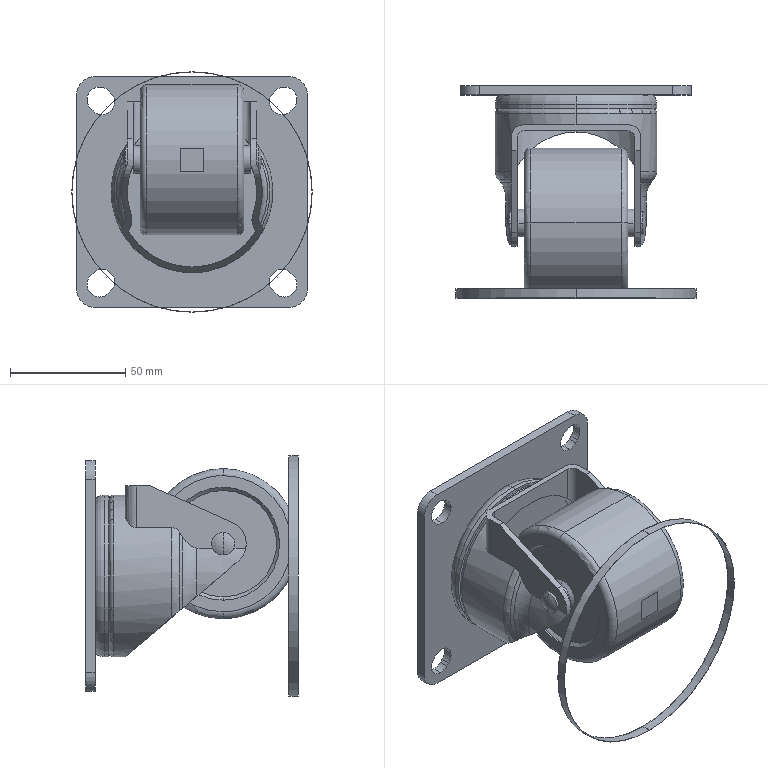Part | NX | features BREP 5 | 5 solids | 130 faces | box 104.2 x 92 x 104.2 mm | volume 222946 mm3 | cylinder 52 | plane 42 | torus 20 | cone 16 | commonest cylinder face diameters 11 x12 10 x6 12 x4 16 x4 49 x4 65 x4